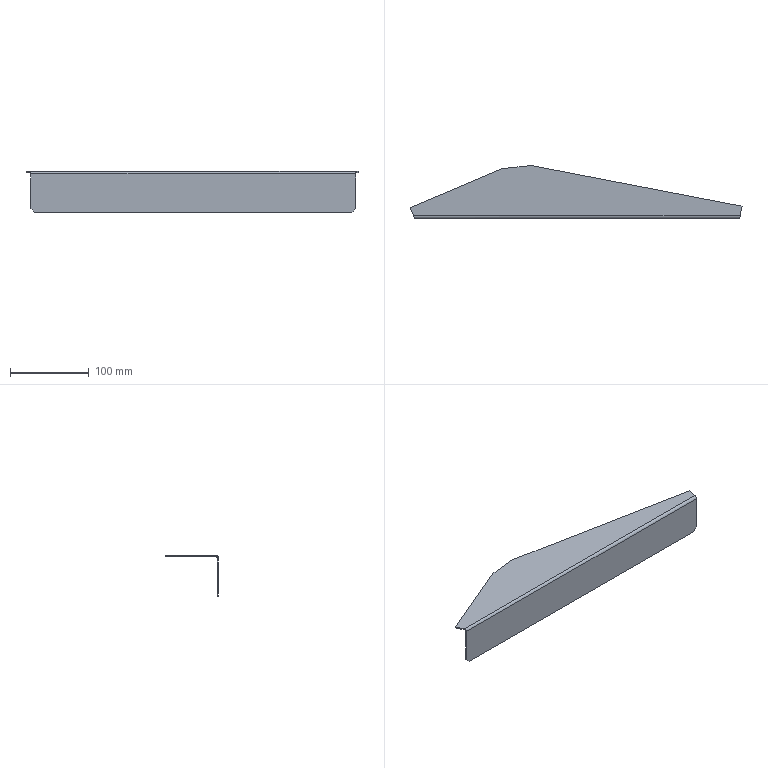Part | SolidWorks | features Chamfer 1, Fillet 1, FlatPattern 1, ICE 1, SMBaseFlange 1, SheetMetal 1 | 1 solid | 24 faces | box 421 x 66.98 x 52 mm | volume 61109 mm3 | plane 14 | spline 6 | cylinder 4 | commonest cylinder face diameters 4 x2 3 x1 6.2 x1
STEP:
#1=CARTESIAN_POINT('',(-56.796,66.969,-1.6));
#2=VERTEX_POINT('',#1);
#3=CARTESIAN_POINT('',(-94.201,63.031,-1.6));
#4=VERTEX_POINT('',#3);
#5=CARTESIAN_POINT('',(200.599,94.063,-1.6));
#6=DIRECTION('',(-0.9945,-0.1047,0.));
#7=VECTOR('',#6,1000.);
#8=LINE('',#5,#7);
#9=EDGE_CURVE('',#2,#4,#8,.T.);
#10=ORIENTED_EDGE('',*,*,#9,.F.);
#11=CARTESIAN_POINT('',(-56.208,66.944,-1.6));
#12=VERTEX_POINT('',#11);
#13=CARTESIAN_POINT('',(-56.587,64.98,-1.6));
#14=DIRECTION('',(0.,0.,-1.));
#15=DIRECTION('',(1.,0.,0.));
#16=AXIS2_PLACEMENT_3D('',#13,#14,#15);
#17=CIRCLE('',#16,2.);
#18=EDGE_CURVE('',#2,#12,#17,.T.);
#19=ORIENTED_EDGE('',*,*,#18,.T.);
#20=CARTESIAN_POINT('',(210.5,15.5,-1.6));
#21=VERTEX_POINT('',#20);
#22=CARTESIAN_POINT('',(213.382,14.944,-1.6));
#23=DIRECTION('',(-0.9819,0.1894,0.));
#24=VECTOR('',#23,1000.);
#25=LINE('',#22,#24);
#26=EDGE_CURVE('',#21,#12,#25,.T.);
#27=ORIENTED_EDGE('',*,*,#26,.F.);
#28=CARTESIAN_POINT('',(208.1,3.1,-1.6));
#29=VERTEX_POINT('',#28);
#30=CARTESIAN_POINT('',(200.008,-38.711,-1.6));
#31=DIRECTION('',(-0.19,-0.9818,0.));
#32=VECTOR('',#31,1000.);
#33=LINE('',#30,#32);
#34=EDGE_CURVE('',#21,#29,#33,.T.);
#35=ORIENTED_EDGE('',*,*,#34,.T.);
#36=CARTESIAN_POINT('',(-205.871,3.1,-1.6));
#37=VERTEX_POINT('',#36);
#38=CARTESIAN_POINT('',(210.5,3.1,-1.6));
#39=DIRECTION('',(-1.,0.,0.));
#40=VECTOR('',#39,1000.);
#41=LINE('',#38,#40);
#42=EDGE_CURVE('',#29,#37,#41,.T.);
#43=ORIENTED_EDGE('',*,*,#42,.T.);
#44=CARTESIAN_POINT('',(-210.5,13.563,-1.6));
#45=VERTEX_POINT('',#44);
#46=CARTESIAN_POINT('',(-136.58,-153.537,-1.6));
#47=DIRECTION('',(-0.4046,0.9145,0.));
#48=VECTOR('',#47,1000.);
#49=LINE('',#46,#48);
#50=EDGE_CURVE('',#37,#45,#49,.T.);
#51=ORIENTED_EDGE('',*,*,#50,.T.);
#52=CARTESIAN_POINT('',(-94.776,62.882,-1.6));
#53=VERTEX_POINT('',#52);
#54=CARTESIAN_POINT('',(140.896,163.321,-1.6));
#55=DIRECTION('',(-0.9199,-0.3921,0.));
#56=VECTOR('',#55,1000.);
#57=LINE('',#54,#56);
#58=EDGE_CURVE('',#53,#45,#57,.T.);
#59=ORIENTED_EDGE('',*,*,#58,.F.);
#60=CARTESIAN_POINT('',(-93.992,61.042,-1.6));
#61=DIRECTION('',(0.,0.,-1.));
#62=DIRECTION('',(1.,0.,0.));
#63=AXIS2_PLACEMENT_3D('',#60,#61,#62);
#64=CIRCLE('',#63,2.);
#65=EDGE_CURVE('',#53,#4,#64,.T.);
#66=ORIENTED_EDGE('',*,*,#65,.T.);
#67=EDGE_LOOP('',(#10,#19,#27,#35,#43,#51,#59,#66));
#68=FACE_OUTER_BOUND('',#67,.T.);
#69=CARTESIAN_POINT('',(210.5,0.,-1.6));
#70=DIRECTION('',(0.,0.,1.));
#71=DIRECTION('',(1.,0.,0.));
#72=AXIS2_PLACEMENT_3D('',#69,#70,#71);
#73=PLANE('',#72);
#74=ADVANCED_FACE('',(#68),#73,.F.);
#75=CARTESIAN_POINT('',(210.5,15.5,0.));
#76=VERTEX_POINT('',#75);
#77=CARTESIAN_POINT('',(-56.208,66.944,0.));
#78=VERTEX_POINT('',#77);
#79=CARTESIAN_POINT('',(213.382,14.944,0.));
#80=DIRECTION('',(-0.9819,0.1894,0.));
#81=VECTOR('',#80,1000.);
#82=LINE('',#79,#81);
#83=EDGE_CURVE('',#76,#78,#82,.T.);
#84=ORIENTED_EDGE('',*,*,#83,.T.);
#85=CARTESIAN_POINT('',(-56.796,66.969,0.));
#86=VERTEX_POINT('',#85);
#87=CARTESIAN_POINT('',(-56.587,64.98,0.));
#88=DIRECTION('',(0.,0.,1.));
#89=DIRECTION('',(1.,0.,0.));
#90=AXIS2_PLACEMENT_3D('',#87,#88,#89);
#91=CIRCLE('',#90,2.);
#92=EDGE_CURVE('',#78,#86,#91,.T.);
#93=ORIENTED_EDGE('',*,*,#92,.T.);
#94=CARTESIAN_POINT('',(-94.201,63.031,0.));
#95=VERTEX_POINT('',#94);
#96=CARTESIAN_POINT('',(200.599,94.063,0.));
#97=DIRECTION('',(-0.9945,-0.1047,0.));
#98=VECTOR('',#97,1000.);
#99=LINE('',#96,#98);
#100=EDGE_CURVE('',#86,#95,#99,.T.);
#101=ORIENTED_EDGE('',*,*,#100,.T.);
#102=CARTESIAN_POINT('',(-94.776,62.882,0.));
#103=VERTEX_POINT('',#102);
#104=CARTESIAN_POINT('',(-93.992,61.042,0.));
#105=DIRECTION('',(0.,0.,1.));
#106=DIRECTION('',(1.,0.,0.));
#107=AXIS2_PLACEMENT_3D('',#104,#105,#106);
#108=CIRCLE('',#107,2.);
#109=EDGE_CURVE('',#95,#103,#108,.T.);
#110=ORIENTED_EDGE('',*,*,#109,.T.);
#111=CARTESIAN_POINT('',(-210.5,13.563,0.));
#112=VERTEX_POINT('',#111);
#113=CARTESIAN_POINT('',(140.896,163.321,0.));
#114=DIRECTION('',(-0.9199,-0.3921,0.));
#115=VECTOR('',#114,1000.);
#116=LINE('',#113,#115);
#117=EDGE_CURVE('',#103,#112,#116,.T.);
#118=ORIENTED_EDGE('',*,*,#117,.T.);
#119=CARTESIAN_POINT('',(-205.871,3.1,0.));
#120=VERTEX_POINT('',#119);
#121=CARTESIAN_POINT('',(-136.58,-153.537,0.));
#122=DIRECTION('',(-0.4046,0.9145,0.));
#123=VECTOR('',#122,1000.);
#124=LINE('',#121,#123);
#125=EDGE_CURVE('',#120,#112,#124,.T.);
#126=ORIENTED_EDGE('',*,*,#125,.F.);
#127=CARTESIAN_POINT('',(208.1,3.1,0.));
#128=VERTEX_POINT('',#127);
#129=CARTESIAN_POINT('',(210.5,3.1,0.));
#130=DIRECTION('',(-1.,0.,0.));
#131=VECTOR('',#130,1000.);
#132=LINE('',#129,#131);
#133=EDGE_CURVE('',#128,#120,#132,.T.);
#134=ORIENTED_EDGE('',*,*,#133,.F.);
#135=CARTESIAN_POINT('',(200.008,-38.711,0.));
#136=DIRECTION('',(-0.19,-0.9818,0.));
#137=VECTOR('',#136,1000.);
#138=LINE('',#135,#137);
#139=EDGE_CURVE('',#76,#128,#138,.T.);
#140=ORIENTED_EDGE('',*,*,#139,.F.);
#141=EDGE_LOOP('',(#84,#93,#101,#110,#118,#126,#134,#140));
#142=FACE_OUTER_BOUND('',#141,.T.);
#143=CARTESIAN_POINT('',(210.5,0.,0.));
#144=DIRECTION('',(0.,0.,1.));
#145=DIRECTION('',(1.,0.,0.));
#146=AXIS2_PLACEMENT_3D('',#143,#144,#145);
#147=PLANE('',#146);
#148=ADVANCED_FACE('',(#142),#147,.T.);
#149=CARTESIAN_POINT('',(207.529,0.09941,-2.321));
#150=VERTEX_POINT('',#149);
#151=CARTESIAN_POINT('',(207.604,0.4379,-1.512));
#152=VERTEX_POINT('',#151);
#153=CARTESIAN_POINT('',(207.529,0.09941,-2.321));
#154=CARTESIAN_POINT('',(207.554,0.1731,-2.037));
#155=CARTESIAN_POINT('',(207.579,0.2875,-1.764));
#156=CARTESIAN_POINT('',(207.604,0.4379,-1.512));
#157=B_SPLINE_CURVE_WITH_KNOTS('',3,(#153,#154,#155,#156),.UNSPECIFIED.,.F.,.F.,(4,4),(0.,1.),.UNSPECIFIED.);
#158=EDGE_CURVE('',#150,#152,#157,.T.);
#159=ORIENTED_EDGE('',*,*,#158,.T.);
#160=CARTESIAN_POINT('',(207.604,0.4379,-1.512));
#161=CARTESIAN_POINT('',(207.645,0.5759,-1.28));
#162=CARTESIAN_POINT('',(207.686,0.7407,-1.072));
#163=CARTESIAN_POINT('',(207.748,1.026,-0.7918));
#164=CARTESIAN_POINT('',(207.769,1.129,-0.7036));
#165=CARTESIAN_POINT('',(207.811,1.343,-0.5427));
#166=CARTESIAN_POINT('',(207.831,1.454,-0.4697));
#167=CARTESIAN_POINT('',(207.893,1.8,-0.273));
#168=CARTESIAN_POINT('',(207.935,2.052,-0.1703));
#169=CARTESIAN_POINT('',(208.017,2.567,-0.03455));
#170=CARTESIAN_POINT('',(208.058,2.831,0.));
#171=CARTESIAN_POINT('',(208.1,3.1,0.));
#172=B_SPLINE_CURVE_WITH_KNOTS('',3,(#160,#161,#162,#163,#164,#165,#166,#167,#168,#169,#170,#171),.UNSPECIFIED.,.F.,.F.,(4,2,2,2,2,4),(0.,0.0008063,0.001209,0.001613,0.002419,0.003225),.UNSPECIFIED.);
#173=EDGE_CURVE('',#152,#128,#172,.T.);
#174=ORIENTED_EDGE('',*,*,#173,.T.);
#175=ORIENTED_EDGE('',*,*,#133,.T.);
#176=CARTESIAN_POINT('',(-204.644,0.2873,-1.797));
#177=VERTEX_POINT('',#176);
#178=CARTESIAN_POINT('',(-205.871,3.1,0.));
#179=CARTESIAN_POINT('',(-205.746,2.812,0.));
#180=CARTESIAN_POINT('',(-205.626,2.529,-0.03947));
#181=CARTESIAN_POINT('',(-205.45,2.113,-0.1577));
#182=CARTESIAN_POINT('',(-205.391,1.975,-0.2075));
#183=CARTESIAN_POINT('',(-205.278,1.71,-0.3255));
#184=CARTESIAN_POINT('',(-205.223,1.582,-0.3934));
#185=CARTESIAN_POINT('',(-205.117,1.335,-0.5473));
#186=CARTESIAN_POINT('',(-205.065,1.217,-0.6333));
#187=CARTESIAN_POINT('',(-204.965,0.9901,-0.824));
#188=CARTESIAN_POINT('',(-204.916,0.8826,-0.9286));
#189=CARTESIAN_POINT('',(-204.826,0.6848,-1.151));
#190=CARTESIAN_POINT('',(-204.784,0.5937,-1.269));
#191=CARTESIAN_POINT('',(-204.707,0.4277,-1.522));
#192=CARTESIAN_POINT('',(-204.672,0.3524,-1.656));
#193=CARTESIAN_POINT('',(-204.644,0.2873,-1.797));
#194=B_SPLINE_CURVE_WITH_KNOTS('',3,(#178,#179,#180,#181,#182,#183,#184,#185,#186,#187,#188,#189,#190,#191,#192,#193),.UNSPECIFIED.,.F.,.F.,(4,2,2,2,2,2,2,4),(0.,0.0009293,0.001394,0.001859,0.002323,0.002788,0.003253,0.003717),.UNSPECIFIED.);
#195=EDGE_CURVE('',#120,#177,#194,.T.);
#196=ORIENTED_EDGE('',*,*,#195,.T.);
#197=CARTESIAN_POINT('',(-204.552,0.07575,-2.419));
#198=VERTEX_POINT('',#197);
#199=CARTESIAN_POINT('',(-204.644,0.2873,-1.797));
#200=CARTESIAN_POINT('',(-204.613,0.195,-1.996));
#201=CARTESIAN_POINT('',(-204.583,0.124,-2.205));
#202=CARTESIAN_POINT('',(-204.552,0.07575,-2.419));
#203=B_SPLINE_CURVE_WITH_KNOTS('',3,(#199,#200,#201,#202),.UNSPECIFIED.,.F.,.F.,(4,4),(0.,1.),.UNSPECIFIED.);
#204=EDGE_CURVE('',#177,#198,#203,.T.);
#205=ORIENTED_EDGE('',*,*,#204,.T.);
#206=CARTESIAN_POINT('',(-204.5,0.,-3.1));
#207=VERTEX_POINT('',#206);
#208=CARTESIAN_POINT('',(-204.552,0.07575,-2.419));
#209=CARTESIAN_POINT('',(-204.535,0.02546,-2.642));
#210=CARTESIAN_POINT('',(-204.517,0.,-2.871));
#211=CARTESIAN_POINT('',(-204.5,0.,-3.1));
#212=B_SPLINE_CURVE_WITH_KNOTS('',3,(#208,#209,#210,#211),.UNSPECIFIED.,.F.,.F.,(4,4),(0.,1.),.UNSPECIFIED.);
#213=EDGE_CURVE('',#198,#207,#212,.T.);
#214=ORIENTED_EDGE('',*,*,#213,.T.);
#215=CARTESIAN_POINT('',(207.5,0.,-3.1));
#216=VERTEX_POINT('',#215);
#217=CARTESIAN_POINT('',(210.5,0.,-3.1));
#218=DIRECTION('',(-1.,0.,0.));
#219=VECTOR('',#218,1000.);
#220=LINE('',#217,#219);
#221=EDGE_CURVE('',#216,#207,#220,.T.);
#222=ORIENTED_EDGE('',*,*,#221,.F.);
#223=CARTESIAN_POINT('',(207.5,0.,-3.1));
#224=CARTESIAN_POINT('',(207.51,0.,-2.838));
#225=CARTESIAN_POINT('',(207.519,0.03349,-2.575));
#226=CARTESIAN_POINT('',(207.529,0.09941,-2.321));
#227=B_SPLINE_CURVE_WITH_KNOTS('',3,(#223,#224,#225,#226),.UNSPECIFIED.,.F.,.F.,(4,4),(0.,1.),.UNSPECIFIED.);
#228=EDGE_CURVE('',#216,#150,#227,.T.);
#229=ORIENTED_EDGE('',*,*,#228,.T.);
#230=EDGE_LOOP('',(#159,#174,#175,#196,#205,#214,#222,#229));
#231=FACE_OUTER_BOUND('',#230,.T.);
#232=CARTESIAN_POINT('',(210.5,3.1,-3.1));
#233=DIRECTION('',(-1.,0.,0.));
#234=DIRECTION('',(0.,0.,1.));
#235=AXIS2_PLACEMENT_3D('',#232,#233,#234);
#236=CYLINDRICAL_SURFACE('',#235,3.1);
#237=ADVANCED_FACE('',(#231),#236,.T.);
#238=CARTESIAN_POINT('',(202.5,0.,-52.));
#239=VERTEX_POINT('',#238);
#240=CARTESIAN_POINT('',(-199.5,0.,-52.));
#241=VERTEX_POINT('',#240);
#242=CARTESIAN_POINT('',(210.5,0.,-52.));
#243=DIRECTION('',(-1.,0.,0.));
#244=VECTOR('',#243,1000.);
#245=LINE('',#242,#244);
#246=EDGE_CURVE('',#239,#241,#245,.T.);
#247=ORIENTED_EDGE('',*,*,#246,.F.);
#248=CARTESIAN_POINT('',(207.5,0.,-47.));
#249=VERTEX_POINT('',#248);
#250=CARTESIAN_POINT('',(232.5,0.,-22.));
#251=DIRECTION('',(0.7071,0.,0.7071));
#252=VECTOR('',#251,1000.);
#253=LINE('',#250,#252);
#254=EDGE_CURVE('',#239,#249,#253,.T.);
#255=ORIENTED_EDGE('',*,*,#254,.T.);
#256=CARTESIAN_POINT('',(207.5,0.,-52.));
#257=DIRECTION('',(0.,0.,1.));
#258=VECTOR('',#257,1000.);
#259=LINE('',#256,#258);
#260=EDGE_CURVE('',#249,#216,#259,.T.);
#261=ORIENTED_EDGE('',*,*,#260,.T.);
#262=ORIENTED_EDGE('',*,*,#221,.T.);
#263=CARTESIAN_POINT('',(-204.5,0.,-47.));
#264=VERTEX_POINT('',#263);
#265=CARTESIAN_POINT('',(-204.5,0.,-52.));
#266=DIRECTION('',(0.,0.,1.));
#267=VECTOR('',#266,1000.);
#268=LINE('',#265,#267);
#269=EDGE_CURVE('',#264,#207,#268,.T.);
#270=ORIENTED_EDGE('',*,*,#269,.F.);
#271=CARTESIAN_POINT('',(-20.5,0.,-231.));
#272=DIRECTION('',(0.7071,0.,-0.7071));
#273=VECTOR('',#272,1000.);
#274=LINE('',#271,#273);
#275=EDGE_CURVE('',#264,#241,#274,.T.);
#276=ORIENTED_EDGE('',*,*,#275,.T.);
#277=EDGE_LOOP('',(#247,#255,#261,#262,#270,#276));
#278=FACE_OUTER_BOUND('',#277,.T.);
#279=CARTESIAN_POINT('',(210.5,0.,0.));
#280=DIRECTION('',(0.,-1.,0.));
#281=DIRECTION('',(0.,0.,-1.));
#282=AXIS2_PLACEMENT_3D('',#279,#280,#281);
#283=PLANE('',#282);
#284=ADVANCED_FACE('',(#278),#283,.T.);
#285=CARTESIAN_POINT('',(202.5,1.6,-52.));
#286=VERTEX_POINT('',#285);
#287=CARTESIAN_POINT('',(-199.5,1.6,-52.));
#288=VERTEX_POINT('',#287);
#289=CARTESIAN_POINT('',(210.5,1.6,-52.));
#290=DIRECTION('',(-1.,0.,0.));
#291=VECTOR('',#290,1000.);
#292=LINE('',#289,#291);
#293=EDGE_CURVE('',#286,#288,#292,.T.);
#294=ORIENTED_EDGE('',*,*,#293,.F.);
#295=CARTESIAN_POINT('',(202.5,1.6,-52.));
#296=DIRECTION('',(0.,-1.,0.));
#297=VECTOR('',#296,1000.);
#298=LINE('',#295,#297);
#299=EDGE_CURVE('',#286,#239,#298,.T.);
#300=ORIENTED_EDGE('',*,*,#299,.T.);
#301=ORIENTED_EDGE('',*,*,#246,.T.);
#302=CARTESIAN_POINT('',(-199.5,1.6,-52.));
#303=DIRECTION('',(0.,1.,0.));
#304=VECTOR('',#303,1000.);
#305=LINE('',#302,#304);
#306=EDGE_CURVE('',#241,#288,#305,.T.);
#307=ORIENTED_EDGE('',*,*,#306,.T.);
#308=EDGE_LOOP('',(#294,#300,#301,#307));
#309=FACE_OUTER_BOUND('',#308,.T.);
#310=CARTESIAN_POINT('',(210.5,1.6,-52.));
#311=DIRECTION('',(0.,0.,-1.));
#312=DIRECTION('',(0.,1.,0.));
#313=AXIS2_PLACEMENT_3D('',#310,#311,#312);
#314=PLANE('',#313);
#315=ADVANCED_FACE('',(#309),#314,.T.);
#316=CARTESIAN_POINT('',(207.5,1.6,-47.));
#317=VERTEX_POINT('',#316);
#318=CARTESIAN_POINT('',(207.5,1.6,-3.1));
#319=VERTEX_POINT('',#318);
#320=CARTESIAN_POINT('',(207.5,1.6,0.));
#321=DIRECTION('',(0.,0.,1.));
#322=VECTOR('',#321,1000.);
#323=LINE('',#320,#322);
#324=EDGE_CURVE('',#317,#319,#323,.T.);
#325=ORIENTED_EDGE('',*,*,#324,.F.);
#326=CARTESIAN_POINT('',(207.5,1.6,-47.));
#327=DIRECTION('',(-0.7071,0.,-0.7071));
#328=VECTOR('',#327,1000.);
#329=LINE('',#326,#328);
#330=EDGE_CURVE('',#317,#286,#329,.T.);
#331=ORIENTED_EDGE('',*,*,#330,.T.);
#332=ORIENTED_EDGE('',*,*,#293,.T.);
#333=CARTESIAN_POINT('',(-204.5,1.6,-47.));
#334=VERTEX_POINT('',#333);
#335=CARTESIAN_POINT('',(-199.5,1.6,-52.));
#336=DIRECTION('',(-0.7071,0.,0.7071));
#337=VECTOR('',#336,1000.);
#338=LINE('',#335,#337);
#339=EDGE_CURVE('',#288,#334,#338,.T.);
#340=ORIENTED_EDGE('',*,*,#339,.T.);
#341=CARTESIAN_POINT('',(-204.5,1.6,-3.1));
#342=VERTEX_POINT('',#341);
#343=CARTESIAN_POINT('',(-204.5,1.6,0.));
#344=DIRECTION('',(0.,0.,1.));
#345=VECTOR('',#344,1000.);
#346=LINE('',#343,#345);
#347=EDGE_CURVE('',#334,#342,#346,.T.);
#348=ORIENTED_EDGE('',*,*,#347,.T.);
#349=CARTESIAN_POINT('',(210.5,1.6,-3.1));
#350=DIRECTION('',(-1.,0.,0.));
#351=VECTOR('',#350,1000.);
#352=LINE('',#349,#351);
#353=EDGE_CURVE('',#319,#342,#352,.T.);
#354=ORIENTED_EDGE('',*,*,#353,.F.);
#355=EDGE_LOOP('',(#325,#331,#332,#340,#348,#354));
#356=FACE_OUTER_BOUND('',#355,.T.);
#357=CARTESIAN_POINT('',(210.5,1.6,0.));
#358=DIRECTION('',(0.,-1.,0.));
#359=DIRECTION('',(0.,0.,-1.));
#360=AXIS2_PLACEMENT_3D('',#357,#358,#359);
#361=PLANE('',#360);
#362=ADVANCED_FACE('',(#356),#361,.F.);
#363=CARTESIAN_POINT('',(207.604,1.812,-2.331));
#364=VERTEX_POINT('',#363);
#365=CARTESIAN_POINT('',(207.604,1.812,-2.331));
#366=CARTESIAN_POINT('',(207.645,1.879,-2.22));
#367=CARTESIAN_POINT('',(207.686,1.958,-2.119));
#368=CARTESIAN_POINT('',(207.769,2.142,-1.938));
#369=CARTESIAN_POINT('',(207.811,2.247,-1.859));
#370=CARTESIAN_POINT('',(207.893,2.471,-1.732));
#371=CARTESIAN_POINT('',(207.934,2.592,-1.683));
#372=CARTESIAN_POINT('',(208.017,2.842,-1.617));
#373=CARTESIAN_POINT('',(208.058,2.97,-1.6));
#374=CARTESIAN_POINT('',(208.1,3.1,-1.6));
#375=B_SPLINE_CURVE_WITH_KNOTS('',3,(#365,#366,#367,#368,#369,#370,#371,#372,#373,#374),.UNSPECIFIED.,.F.,.F.,(4,2,2,2,4),(0.000000002,0.0004046,0.0008091,0.001214,0.001618),.UNSPECIFIED.);
#376=EDGE_CURVE('',#364,#29,#375,.T.);
#377=ORIENTED_EDGE('',*,*,#376,.F.);
#378=CARTESIAN_POINT('',(207.529,1.648,-2.723));
#379=VERTEX_POINT('',#378);
#380=CARTESIAN_POINT('',(207.529,1.648,-2.723));
#381=CARTESIAN_POINT('',(207.554,1.684,-2.586));
#382=CARTESIAN_POINT('',(207.579,1.739,-2.453));
#383=CARTESIAN_POINT('',(207.604,1.812,-2.331));
#384=B_SPLINE_CURVE_WITH_KNOTS('',3,(#380,#381,#382,#383),.UNSPECIFIED.,.F.,.F.,(4,4),(0.000005952,1.),.UNSPECIFIED.);
#385=EDGE_CURVE('',#379,#364,#384,.T.);
#386=ORIENTED_EDGE('',*,*,#385,.F.);
#387=CARTESIAN_POINT('',(207.5,1.6,-3.1));
#388=CARTESIAN_POINT('',(207.51,1.6,-2.973));
#389=CARTESIAN_POINT('',(207.519,1.616,-2.846));
#390=CARTESIAN_POINT('',(207.529,1.648,-2.723));
#391=B_SPLINE_CURVE_WITH_KNOTS('',3,(#387,#388,#389,#390),.UNSPECIFIED.,.F.,.F.,(4,4),(0.,1.),.UNSPECIFIED.);
#392=EDGE_CURVE('',#319,#379,#391,.T.);
#393=ORIENTED_EDGE('',*,*,#392,.F.);
#394=ORIENTED_EDGE('',*,*,#353,.T.);
#395=CARTESIAN_POINT('',(-204.552,1.637,-2.77));
#396=VERTEX_POINT('',#395);
#397=CARTESIAN_POINT('',(-204.552,1.637,-2.77));
#398=CARTESIAN_POINT('',(-204.535,1.612,-2.878));
#399=CARTESIAN_POINT('',(-204.517,1.6,-2.989));
#400=CARTESIAN_POINT('',(-204.5,1.6,-3.1));
#401=B_SPLINE_CURVE_WITH_KNOTS('',3,(#397,#398,#399,#400),.UNSPECIFIED.,.F.,.F.,(4,4),(0.000005695,1.),.UNSPECIFIED.);
#402=EDGE_CURVE('',#396,#342,#401,.T.);
#403=ORIENTED_EDGE('',*,*,#402,.F.);
#404=CARTESIAN_POINT('',(-204.644,1.739,-2.469));
#405=VERTEX_POINT('',#404);
#406=CARTESIAN_POINT('',(-204.644,1.739,-2.469));
#407=CARTESIAN_POINT('',(-204.613,1.694,-2.566));
#408=CARTESIAN_POINT('',(-204.583,1.66,-2.667));
#409=CARTESIAN_POINT('',(-204.552,1.637,-2.77));
#410=B_SPLINE_CURVE_WITH_KNOTS('',3,(#406,#407,#408,#409),.UNSPECIFIED.,.F.,.F.,(4,4),(0.,1.),.UNSPECIFIED.);
#411=EDGE_CURVE('',#405,#396,#410,.T.);
#412=ORIENTED_EDGE('',*,*,#411,.F.);
#413=CARTESIAN_POINT('',(-205.871,3.1,-1.6));
#414=CARTESIAN_POINT('',(-205.753,2.968,-1.6));
#415=CARTESIAN_POINT('',(-205.637,2.837,-1.617));
#416=CARTESIAN_POINT('',(-205.411,2.578,-1.687));
#417=CARTESIAN_POINT('',(-205.299,2.45,-1.741));
#418=CARTESIAN_POINT('',(-205.086,2.211,-1.884));
#419=CARTESIAN_POINT('',(-204.983,2.098,-1.974));
#420=CARTESIAN_POINT('',(-204.793,1.896,-2.193));
#421=CARTESIAN_POINT('',(-204.707,1.809,-2.317));
#422=CARTESIAN_POINT('',(-204.644,1.739,-2.469));
#423=B_SPLINE_CURVE_WITH_KNOTS('',3,(#413,#414,#415,#416,#417,#418,#419,#420,#421,#422),.UNSPECIFIED.,.F.,.F.,(4,2,2,2,4),(0.,0.0005259,0.001052,0.001578,0.002104),.UNSPECIFIED.);
#424=EDGE_CURVE('',#37,#405,#423,.T.);
#425=ORIENTED_EDGE('',*,*,#424,.F.);
#426=ORIENTED_EDGE('',*,*,#42,.F.);
#427=EDGE_LOOP('',(#377,#386,#393,#394,#403,#412,#425,#426));
#428=FACE_OUTER_BOUND('',#427,.T.);
#429=CARTESIAN_POINT('',(210.5,3.1,-3.1));
#430=DIRECTION('',(-1.,0.,0.));
#431=DIRECTION('',(0.,0.,1.));
#432=AXIS2_PLACEMENT_3D('',#429,#430,#431);
#433=CYLINDRICAL_SURFACE('',#432,1.5);
#434=ADVANCED_FACE('',(#428),#433,.F.);
#435=CARTESIAN_POINT('',(-204.552,0.8484,-2.593));
#436=DIRECTION('',(0.,-0.9756,0.2197));
#437=VECTOR('',#436,1000.);
#438=LINE('',#435,#437);
#439=EDGE_CURVE('',#396,#198,#438,.T.);
#440=ORIENTED_EDGE('',*,*,#439,.F.);
#441=ORIENTED_EDGE('',*,*,#402,.T.);
#442=CARTESIAN_POINT('',(-204.5,0.,-3.1));
#443=DIRECTION('',(0.,1.,0.));
#444=VECTOR('',#443,1000.);
#445=LINE('',#442,#444);
#446=EDGE_CURVE('',#207,#342,#445,.T.);
#447=ORIENTED_EDGE('',*,*,#446,.F.);
#448=ORIENTED_EDGE('',*,*,#213,.F.);
#449=EDGE_LOOP('',(#440,#441,#447,#448));
#450=FACE_OUTER_BOUND('',#449,.T.);
#451=CARTESIAN_POINT('',(-204.552,0.06014,-2.415));
#452=CARTESIAN_POINT('',(-204.535,0.009586,-2.64));
#453=CARTESIAN_POINT('',(-204.517,-0.016,-2.87));
#454=CARTESIAN_POINT('',(-204.5,-0.016,-3.1));
#455=CARTESIAN_POINT('',(-204.552,0.07575,-2.419));
#456=CARTESIAN_POINT('',(-204.535,0.02545,-2.642));
#457=CARTESIAN_POINT('',(-204.517,0.,-2.871));
#458=CARTESIAN_POINT('',(-204.5,0.,-3.1));
#459=CARTESIAN_POINT('',(-204.552,1.637,-2.77));
#460=CARTESIAN_POINT('',(-204.535,1.612,-2.878));
#461=CARTESIAN_POINT('',(-204.517,1.6,-2.989));
#462=CARTESIAN_POINT('',(-204.5,1.6,-3.1));
#463=B_SPLINE_SURFACE_WITH_KNOTS('',1,3,((#451,#452,#453,#454),(#455,#456,#457,#458),(#459,#460,#461,#462)),.UNSPECIFIED.,.F.,.F.,.F.,(2,1,2),(4,4),(-0.01,0.,1.),(0.,1.),.UNSPECIFIED.);
#464=ADVANCED_FACE('',(#450),#463,.T.);
#465=CARTESIAN_POINT('',(-204.644,1.006,-2.13));
#466=DIRECTION('',(0.,-0.9073,0.4204));
#467=VECTOR('',#466,1000.);
#468=LINE('',#465,#467);
#469=EDGE_CURVE('',#405,#177,#468,.T.);
#470=ORIENTED_EDGE('',*,*,#469,.F.);
#471=ORIENTED_EDGE('',*,*,#411,.T.);
#472=ORIENTED_EDGE('',*,*,#439,.T.);
#473=ORIENTED_EDGE('',*,*,#204,.F.);
#474=EDGE_LOOP('',(#470,#471,#472,#473));
#475=FACE_OUTER_BOUND('',#474,.T.);
#476=CARTESIAN_POINT('',(-204.644,0.2727,-1.79));
#477=CARTESIAN_POINT('',(-204.613,0.18,-1.99));
#478=CARTESIAN_POINT('',(-204.583,0.1086,-2.2));
#479=CARTESIAN_POINT('',(-204.552,0.06014,-2.415));
#480=CARTESIAN_POINT('',(-204.644,0.2873,-1.797));
#481=CARTESIAN_POINT('',(-204.613,0.195,-1.996));
#482=CARTESIAN_POINT('',(-204.583,0.124,-2.205));
#483=CARTESIAN_POINT('',(-204.552,0.07575,-2.419));
#484=CARTESIAN_POINT('',(-204.644,1.739,-2.469));
#485=CARTESIAN_POINT('',(-204.613,1.694,-2.566));
#486=CARTESIAN_POINT('',(-204.583,1.66,-2.667));
#487=CARTESIAN_POINT('',(-204.552,1.637,-2.77));
#488=B_SPLINE_SURFACE_WITH_KNOTS('',1,3,((#476,#477,#478,#479),(#480,#481,#482,#483),(#484,#485,#486,#487)),.UNSPECIFIED.,.F.,.F.,.F.,(2,1,2),(4,4),(-0.01,0.,1.),(0.,1.),.UNSPECIFIED.);
#489=ADVANCED_FACE('',(#475),#488,.T.);
#490=CARTESIAN_POINT('',(-205.871,3.1,-1.6));
#491=DIRECTION('',(0.,0.,-1.));
#492=VECTOR('',#491,1000.);
#493=LINE('',#490,#492);
#494=EDGE_CURVE('',#120,#37,#493,.T.);
#495=ORIENTED_EDGE('',*,*,#494,.T.);
#496=ORIENTED_EDGE('',*,*,#424,.T.);
#497=ORIENTED_EDGE('',*,*,#469,.T.);
#498=ORIENTED_EDGE('',*,*,#195,.F.);
#499=EDGE_LOOP('',(#495,#496,#497,#498));
#500=FACE_OUTER_BOUND('',#499,.T.);
#501=CARTESIAN_POINT('',(-205.871,3.1,0.016));
#502=CARTESIAN_POINT('',(-205.703,2.712,0.016));
#503=CARTESIAN_POINT('',(-205.552,2.35,-0.05635));
#504=CARTESIAN_POINT('',(-205.282,1.71,-0.2906));
#505=CARTESIAN_POINT('',(-205.163,1.431,-0.4522));
#506=CARTESIAN_POINT('',(-204.958,0.9634,-0.8127));
#507=CARTESIAN_POINT('',(-204.872,0.774,-1.012));
#508=CARTESIAN_POINT('',(-204.734,0.4716,-1.408));
#509=CARTESIAN_POINT('',(-204.681,0.3582,-1.606));
#510=CARTESIAN_POINT('',(-204.644,0.2727,-1.79));
#511=CARTESIAN_POINT('',(-205.871,3.1,0.));
#512=CARTESIAN_POINT('',(-205.703,2.714,0.));
#513=CARTESIAN_POINT('',(-205.552,2.354,-0.07198));
#514=CARTESIAN_POINT('',(-205.282,1.717,-0.3051));
#515=CARTESIAN_POINT('',(-205.163,1.44,-0.4658));
#516=CARTESIAN_POINT('',(-204.958,0.9744,-0.8244));
#517=CARTESIAN_POINT('',(-204.872,0.786,-1.022));
#518=CARTESIAN_POINT('',(-204.734,0.4851,-1.417));
#519=CARTESIAN_POINT('',(-204.681,0.3722,-1.613));
#520=CARTESIAN_POINT('',(-204.644,0.2873,-1.797));
#521=CARTESIAN_POINT('',(-205.871,3.1,-1.6));
#522=CARTESIAN_POINT('',(-205.703,2.914,-1.6));
#523=CARTESIAN_POINT('',(-205.552,2.739,-1.635));
#524=CARTESIAN_POINT('',(-205.282,2.431,-1.748));
#525=CARTESIAN_POINT('',(-205.163,2.297,-1.825));
#526=CARTESIAN_POINT('',(-204.958,2.071,-1.999));
#527=CARTESIAN_POINT('',(-204.872,1.98,-2.095));
#528=CARTESIAN_POINT('',(-204.734,1.835,-2.285));
#529=CARTESIAN_POINT('',(-204.681,1.78,-2.381));
#530=CARTESIAN_POINT('',(-204.644,1.739,-2.469));
#531=CARTESIAN_POINT('',(-205.871,3.1,-1.616));
#532=CARTESIAN_POINT('',(-205.703,2.916,-1.616));
#533=CARTESIAN_POINT('',(-205.552,2.743,-1.651));
#534=CARTESIAN_POINT('',(-205.282,2.438,-1.762));
#535=CARTESIAN_POINT('',(-205.163,2.305,-1.839));
#536=CARTESIAN_POINT('',(-204.958,2.083,-2.011));
#537=CARTESIAN_POINT('',(-204.872,1.992,-2.105));
#538=CARTESIAN_POINT('',(-204.734,1.848,-2.294));
#539=CARTESIAN_POINT('',(-204.681,1.794,-2.388));
#540=CARTESIAN_POINT('',(-204.644,1.754,-2.476));
#541=B_SPLINE_SURFACE_WITH_KNOTS('',1,3,((#501,#502,#503,#504,#505,#506,#507,#508,#509,#510),(#511,#512,#513,#514,#515,#516,#517,#518,#519,#520),(#521,#522,#523,#524,#525,#526,#527,#528,#529,#530),(#531,#532,#533,#534,#535,#536,#537,#538,#539,#540)),.UNSPECIFIED.,.F.,.F.,.F.,(2,1,1,2),(4,2,2,2,4),(-0.01,0.,1.,1.01),(0.,0.25,0.5,0.75,1.),.UNSPECIFIED.);
#542=ADVANCED_FACE('',(#500),#541,.T.);
#543=CARTESIAN_POINT('',(-210.5,13.563,0.));
#544=DIRECTION('',(0.,0.,1.));
#545=VECTOR('',#544,1000.);
#546=LINE('',#543,#545);
#547=EDGE_CURVE('',#45,#112,#546,.T.);
#548=ORIENTED_EDGE('',*,*,#547,.F.);
#549=ORIENTED_EDGE('',*,*,#50,.F.);
#550=ORIENTED_EDGE('',*,*,#494,.F.);
#551=ORIENTED_EDGE('',*,*,#125,.T.);
#552=EDGE_LOOP('',(#548,#549,#550,#551));
#553=FACE_OUTER_BOUND('',#552,.T.);
#554=CARTESIAN_POINT('',(-136.58,-153.537,-1.6));
#555=DIRECTION('',(0.9145,0.4046,0.));
#556=DIRECTION('',(-0.4046,0.9145,0.));
#557=AXIS2_PLACEMENT_3D('',#554,#555,#556);
#558=PLANE('',#557);
#559=ADVANCED_FACE('',(#553),#558,.F.);
#560=ORIENTED_EDGE('',*,*,#347,.F.);
#561=CARTESIAN_POINT('',(-204.5,0.,-47.));
#562=DIRECTION('',(0.,-1.,0.));
#563=VECTOR('',#562,1000.);
#564=LINE('',#561,#563);
#565=EDGE_CURVE('',#334,#264,#564,.T.);
#566=ORIENTED_EDGE('',*,*,#565,.T.);
#567=ORIENTED_EDGE('',*,*,#269,.T.);
#568=ORIENTED_EDGE('',*,*,#446,.T.);
#569=EDGE_LOOP('',(#560,#566,#567,#568));
#570=FACE_OUTER_BOUND('',#569,.T.);
#571=CARTESIAN_POINT('',(-204.5,0.,-52.));
#572=DIRECTION('',(1.,0.,0.));
#573=DIRECTION('',(0.,0.,1.));
#574=AXIS2_PLACEMENT_3D('',#571,#572,#573);
#575=PLANE('',#574);
#576=ADVANCED_FACE('',(#570),#575,.F.);
#577=ORIENTED_EDGE('',*,*,#26,.T.);
#578=CARTESIAN_POINT('',(-56.208,66.944,0.));
#579=DIRECTION('',(0.,0.,1.));
#580=VECTOR('',#579,1000.);
#581=LINE('',#578,#580);
#582=EDGE_CURVE('',#12,#78,#581,.T.);
#583=ORIENTED_EDGE('',*,*,#582,.T.);
#584=ORIENTED_EDGE('',*,*,#83,.F.);
#585=CARTESIAN_POINT('',(210.5,15.5,0.));
#586=DIRECTION('',(0.,0.,1.));
#587=VECTOR('',#586,1000.);
#588=LINE('',#585,#587);
#589=EDGE_CURVE('',#21,#76,#588,.T.);
#590=ORIENTED_EDGE('',*,*,#589,.F.);
#591=EDGE_LOOP('',(#577,#583,#584,#590));
#592=FACE_OUTER_BOUND('',#591,.T.);
#593=CARTESIAN_POINT('',(213.382,14.944,0.));
#594=DIRECTION('',(-0.1894,-0.9819,0.));
#595=DIRECTION('',(-0.9819,0.1894,0.));
#596=AXIS2_PLACEMENT_3D('',#593,#594,#595);
#597=PLANE('',#596);
#598=ADVANCED_FACE('',(#592),#597,.F.);
#599=ORIENTED_EDGE('',*,*,#100,.F.);
#600=CARTESIAN_POINT('',(-56.796,66.969,0.));
#601=DIRECTION('',(0.,0.,-1.));
#602=VECTOR('',#601,1000.);
#603=LINE('',#600,#602);
#604=EDGE_CURVE('',#86,#2,#603,.T.);
#605=ORIENTED_EDGE('',*,*,#604,.T.);
#606=ORIENTED_EDGE('',*,*,#9,.T.);
#607=CARTESIAN_POINT('',(-94.201,63.031,0.));
#608=DIRECTION('',(0.,0.,1.));
#609=VECTOR('',#608,1000.);
#610=LINE('',#607,#609);
#611=EDGE_CURVE('',#4,#95,#610,.T.);
#612=ORIENTED_EDGE('',*,*,#611,.T.);
#613=EDGE_LOOP('',(#599,#605,#606,#612));
#614=FACE_OUTER_BOUND('',#613,.T.);
#615=CARTESIAN_POINT('',(200.599,94.063,0.));
#616=DIRECTION('',(0.1047,-0.9945,0.));
#617=DIRECTION('',(-0.9945,-0.1047,0.));
#618=AXIS2_PLACEMENT_3D('',#615,#616,#617);
#619=PLANE('',#618);
#620=ADVANCED_FACE('',(#614),#619,.F.);
#621=ORIENTED_EDGE('',*,*,#117,.F.);
#622=CARTESIAN_POINT('',(-94.776,62.882,0.));
#623=DIRECTION('',(0.,0.,-1.));
#624=VECTOR('',#623,1000.);
#625=LINE('',#622,#624);
#626=EDGE_CURVE('',#103,#53,#625,.T.);
#627=ORIENTED_EDGE('',*,*,#626,.T.);
#628=ORIENTED_EDGE('',*,*,#58,.T.);
#629=ORIENTED_EDGE('',*,*,#547,.T.);
#630=EDGE_LOOP('',(#621,#627,#628,#629));
#631=FACE_OUTER_BOUND('',#630,.T.);
#632=CARTESIAN_POINT('',(140.896,163.321,0.));
#633=DIRECTION('',(0.3921,-0.9199,0.));
#634=DIRECTION('',(-0.9199,-0.3921,0.));
#635=AXIS2_PLACEMENT_3D('',#632,#633,#634);
#636=PLANE('',#635);
#637=ADVANCED_FACE('',(#631),#636,.F.);
#638=CARTESIAN_POINT('',(207.604,1.118,-1.917));
#639=DIRECTION('',(0.,-0.8588,0.5124));
#640=VECTOR('',#639,1000.);
#641=LINE('',#638,#640);
#642=EDGE_CURVE('',#364,#152,#641,.T.);
#643=ORIENTED_EDGE('',*,*,#642,.F.);
#644=ORIENTED_EDGE('',*,*,#376,.T.);
#645=CARTESIAN_POINT('',(208.1,3.1,0.));
#646=DIRECTION('',(0.,0.,-1.));
#647=VECTOR('',#646,1000.);
#648=LINE('',#645,#647);
#649=EDGE_CURVE('',#128,#29,#648,.T.);
#650=ORIENTED_EDGE('',*,*,#649,.F.);
#651=ORIENTED_EDGE('',*,*,#173,.F.);
#652=EDGE_LOOP('',(#643,#644,#650,#651));
#653=FACE_OUTER_BOUND('',#652,.T.);
#654=CARTESIAN_POINT('',(207.599,0.4076,-1.531));
#655=CARTESIAN_POINT('',(207.6,0.4131,-1.522));
#656=CARTESIAN_POINT('',(207.602,0.4186,-1.513));
#657=CARTESIAN_POINT('',(207.604,0.4241,-1.503));
#658=CARTESIAN_POINT('',(207.686,0.6991,-1.043));
#659=CARTESIAN_POINT('',(207.769,1.095,-0.6552));
#660=CARTESIAN_POINT('',(207.935,2.028,-0.1255));
#661=CARTESIAN_POINT('',(208.017,2.563,0.016));
#662=CARTESIAN_POINT('',(208.1,3.1,0.016));
#663=CARTESIAN_POINT('',(207.599,0.4215,-1.539));
#664=CARTESIAN_POINT('',(207.6,0.4269,-1.53));
#665=CARTESIAN_POINT('',(207.602,0.4324,-1.521));
#666=CARTESIAN_POINT('',(207.604,0.4379,-1.512));
#667=CARTESIAN_POINT('',(207.686,0.7114,-1.053));
#668=CARTESIAN_POINT('',(207.769,1.105,-0.6677));
#669=CARTESIAN_POINT('',(207.935,2.033,-0.1408));
#670=CARTESIAN_POINT('',(208.017,2.566,0.));
#671=CARTESIAN_POINT('',(208.1,3.1,0.));
#672=CARTESIAN_POINT('',(207.599,1.804,-2.345));
#673=CARTESIAN_POINT('',(207.6,1.807,-2.34));
#674=CARTESIAN_POINT('',(207.602,1.809,-2.336));
#675=CARTESIAN_POINT('',(207.604,1.812,-2.331));
#676=CARTESIAN_POINT('',(207.686,1.944,-2.11));
#677=CARTESIAN_POINT('',(207.769,2.135,-1.923));
#678=CARTESIAN_POINT('',(207.935,2.584,-1.668));
#679=CARTESIAN_POINT('',(208.017,2.842,-1.6));
#680=CARTESIAN_POINT('',(208.1,3.1,-1.6));
#681=B_SPLINE_SURFACE_WITH_KNOTS('',1,3,((#654,#655,#656,#657,#658,#659,#660,#661,#662),(#663,#664,#665,#666,#667,#668,#669,#670,#671),(#672,#673,#674,#675,#676,#677,#678,#679,#680)),.UNSPECIFIED.,.F.,.F.,.F.,(2,1,2),(4,3,2,4),(-0.01,0.,1.),(-0.01,0.,0.5,1.),.UNSPECIFIED.);
#682=ADVANCED_FACE('',(#653),#681,.T.);
#683=CARTESIAN_POINT('',(207.529,0.8738,-2.522));
#684=DIRECTION('',(0.,-0.9679,0.2512));
#685=VECTOR('',#684,1000.);
#686=LINE('',#683,#685);
#687=EDGE_CURVE('',#379,#150,#686,.T.);
#688=ORIENTED_EDGE('',*,*,#687,.F.);
#689=ORIENTED_EDGE('',*,*,#385,.T.);
#690=ORIENTED_EDGE('',*,*,#642,.T.);
#691=ORIENTED_EDGE('',*,*,#158,.F.);
#692=EDGE_LOOP('',(#688,#689,#690,#691));
#693=FACE_OUTER_BOUND('',#692,.T.);
#694=CARTESIAN_POINT('',(207.529,0.08392,-2.317));
#695=CARTESIAN_POINT('',(207.554,0.158,-2.032));
#696=CARTESIAN_POINT('',(207.579,0.2729,-1.757));
#697=CARTESIAN_POINT('',(207.604,0.4241,-1.503));
#698=CARTESIAN_POINT('',(207.529,0.09941,-2.321));
#699=CARTESIAN_POINT('',(207.554,0.1732,-2.037));
#700=CARTESIAN_POINT('',(207.579,0.2875,-1.764));
#701=CARTESIAN_POINT('',(207.604,0.4379,-1.512));
#702=CARTESIAN_POINT('',(207.529,1.648,-2.723));
#703=CARTESIAN_POINT('',(207.554,1.684,-2.586));
#704=CARTESIAN_POINT('',(207.579,1.739,-2.453));
#705=CARTESIAN_POINT('',(207.604,1.812,-2.331));
#706=CARTESIAN_POINT('',(207.529,1.664,-2.727));
#707=CARTESIAN_POINT('',(207.554,1.699,-2.591));
#708=CARTESIAN_POINT('',(207.579,1.754,-2.46));
#709=CARTESIAN_POINT('',(207.604,1.826,-2.34));
#710=B_SPLINE_SURFACE_WITH_KNOTS('',1,3,((#694,#695,#696,#697),(#698,#699,#700,#701),(#702,#703,#704,#705),(#706,#707,#708,#709)),.UNSPECIFIED.,.F.,.F.,.F.,(2,1,1,2),(4,4),(-0.01,0.,1.,1.01),(0.000000407,1.),.UNSPECIFIED.);
#711=ADVANCED_FACE('',(#693),#710,.T.);
#712=CARTESIAN_POINT('',(207.5,0.,-3.1));
#713=DIRECTION('',(0.,1.,0.));
#714=VECTOR('',#713,1000.);
#715=LINE('',#712,#714);
#716=EDGE_CURVE('',#216,#319,#715,.T.);
#717=ORIENTED_EDGE('',*,*,#716,.T.);
#718=ORIENTED_EDGE('',*,*,#392,.T.);
#719=ORIENTED_EDGE('',*,*,#687,.T.);
#720=ORIENTED_EDGE('',*,*,#228,.F.);
#721=EDGE_LOOP('',(#717,#718,#719,#720));
#722=FACE_OUTER_BOUND('',#721,.T.);
#723=CARTESIAN_POINT('',(207.5,-0.016,-3.1));
#724=CARTESIAN_POINT('',(207.51,-0.016,-2.836));
#725=CARTESIAN_POINT('',(207.519,0.01766,-2.573));
#726=CARTESIAN_POINT('',(207.529,0.08392,-2.317));
#727=CARTESIAN_POINT('',(207.5,0.,-3.1));
#728=CARTESIAN_POINT('',(207.51,0.,-2.838));
#729=CARTESIAN_POINT('',(207.519,0.03348,-2.575));
#730=CARTESIAN_POINT('',(207.529,0.09941,-2.321));
#731=CARTESIAN_POINT('',(207.5,1.6,-3.1));
#732=CARTESIAN_POINT('',(207.51,1.6,-2.973));
#733=CARTESIAN_POINT('',(207.519,1.616,-2.846));
#734=CARTESIAN_POINT('',(207.529,1.648,-2.723));
#735=B_SPLINE_SURFACE_WITH_KNOTS('',1,3,((#723,#724,#725,#726),(#727,#728,#729,#730),(#731,#732,#733,#734)),.UNSPECIFIED.,.F.,.F.,.F.,(2,1,2),(4,4),(-0.01,0.,1.),(0.,1.),.UNSPECIFIED.);
#736=ADVANCED_FACE('',(#722),#735,.T.);
#737=ORIENTED_EDGE('',*,*,#139,.T.);
#738=ORIENTED_EDGE('',*,*,#649,.T.);
#739=ORIENTED_EDGE('',*,*,#34,.F.);
#740=ORIENTED_EDGE('',*,*,#589,.T.);
#741=EDGE_LOOP('',(#737,#738,#739,#740));
#742=FACE_OUTER_BOUND('',#741,.T.);
#743=CARTESIAN_POINT('',(200.008,-38.711,0.));
#744=DIRECTION('',(-0.9818,0.19,0.));
#745=DIRECTION('',(-0.19,-0.9818,0.));
#746=AXIS2_PLACEMENT_3D('',#743,#744,#745);
#747=PLANE('',#746);
#748=ADVANCED_FACE('',(#742),#747,.F.);
#749=ORIENTED_EDGE('',*,*,#260,.F.);
#750=CARTESIAN_POINT('',(207.5,0.,-47.));
#751=DIRECTION('',(0.,1.,0.));
#752=VECTOR('',#751,1000.);
#753=LINE('',#750,#752);
#754=EDGE_CURVE('',#249,#317,#753,.T.);
#755=ORIENTED_EDGE('',*,*,#754,.T.);
#756=ORIENTED_EDGE('',*,*,#324,.T.);
#757=ORIENTED_EDGE('',*,*,#716,.F.);
#758=EDGE_LOOP('',(#749,#755,#756,#757));
#759=FACE_OUTER_BOUND('',#758,.T.);
#760=CARTESIAN_POINT('',(207.5,0.,-52.));
#761=DIRECTION('',(1.,0.,0.));
#762=DIRECTION('',(0.,0.,1.));
#763=AXIS2_PLACEMENT_3D('',#760,#761,#762);
#764=PLANE('',#763);
#765=ADVANCED_FACE('',(#759),#764,.T.);
#766=ORIENTED_EDGE('',*,*,#254,.F.);
#767=ORIENTED_EDGE('',*,*,#299,.F.);
#768=ORIENTED_EDGE('',*,*,#330,.F.);
#769=ORIENTED_EDGE('',*,*,#754,.F.);
#770=EDGE_LOOP('',(#766,#767,#768,#769));
#771=FACE_OUTER_BOUND('',#770,.T.);
#772=CARTESIAN_POINT('',(207.5,0.,-47.));
#773=DIRECTION('',(-0.7071,0.,0.7071));
#774=DIRECTION('',(0.,1.,0.));
#775=AXIS2_PLACEMENT_3D('',#772,#773,#774);
#776=PLANE('',#775);
#777=ADVANCED_FACE('',(#771),#776,.F.);
#778=ORIENTED_EDGE('',*,*,#275,.F.);
#779=ORIENTED_EDGE('',*,*,#565,.F.);
#780=ORIENTED_EDGE('',*,*,#339,.F.);
#781=ORIENTED_EDGE('',*,*,#306,.F.);
#782=EDGE_LOOP('',(#778,#779,#780,#781));
#783=FACE_OUTER_BOUND('',#782,.T.);
#784=CARTESIAN_POINT('',(-199.5,1.6,-52.));
#785=DIRECTION('',(-0.7071,0.,-0.7071));
#786=DIRECTION('',(0.,-1.,0.));
#787=AXIS2_PLACEMENT_3D('',#784,#785,#786);
#788=PLANE('',#787);
#789=ADVANCED_FACE('',(#783),#788,.T.);
#790=ORIENTED_EDGE('',*,*,#18,.F.);
#791=ORIENTED_EDGE('',*,*,#604,.F.);
#792=ORIENTED_EDGE('',*,*,#92,.F.);
#793=ORIENTED_EDGE('',*,*,#582,.F.);
#794=EDGE_LOOP('',(#790,#791,#792,#793));
#795=FACE_OUTER_BOUND('',#794,.T.);
#796=CARTESIAN_POINT('',(-56.587,64.98,0.));
#797=DIRECTION('',(0.,0.,1.));
#798=DIRECTION('',(1.,0.,0.));
#799=AXIS2_PLACEMENT_3D('',#796,#797,#798);
#800=CYLINDRICAL_SURFACE('',#799,2.);
#801=ADVANCED_FACE('',(#795),#800,.T.);
#802=ORIENTED_EDGE('',*,*,#65,.F.);
#803=ORIENTED_EDGE('',*,*,#626,.F.);
#804=ORIENTED_EDGE('',*,*,#109,.F.);
#805=ORIENTED_EDGE('',*,*,#611,.F.);
#806=EDGE_LOOP('',(#802,#803,#804,#805));
#807=FACE_OUTER_BOUND('',#806,.T.);
#808=CARTESIAN_POINT('',(-93.992,61.042,0.));
#809=DIRECTION('',(0.,0.,1.));
#810=DIRECTION('',(1.,0.,0.));
#811=AXIS2_PLACEMENT_3D('',#808,#809,#810);
#812=CYLINDRICAL_SURFACE('',#811,2.);
#813=ADVANCED_FACE('',(#807),#812,.T.);
#814=CLOSED_SHELL('',(#74,#148,#237,#284,#315,#362,#434,#464,#489,#542,#559,#576,#598,#620,#637,#682,#711,#736,#748,#765,#777,#789,#801,#813));
#815=MANIFOLD_SOLID_BREP('',#814);
#816=CARTESIAN_POINT('',(0.,0.,0.));
#817=DIRECTION('',(0.,0.,1.));
#818=DIRECTION('',(1.,0.,0.));
#819=AXIS2_PLACEMENT_3D('',#816,#817,#818);
#820=(LENGTH_UNIT()NAMED_UNIT(*)SI_UNIT(.MILLI.,.METRE.));
#821=UNCERTAINTY_MEASURE_WITH_UNIT(LENGTH_MEASURE(0.00001),#820,'','');
#822=(NAMED_UNIT(*)PLANE_ANGLE_UNIT()SI_UNIT($,.RADIAN.));
#823=(NAMED_UNIT(*)SI_UNIT($,.STERADIAN.)SOLID_ANGLE_UNIT());
#824=(GEOMETRIC_REPRESENTATION_CONTEXT(3)GLOBAL_UNCERTAINTY_ASSIGNED_CONTEXT((#821))GLOBAL_UNIT_ASSIGNED_CONTEXT((#820,#822,#823))REPRESENTATION_CONTEXT('',''));
#825=ADVANCED_BREP_SHAPE_REPRESENTATION('',(#815,#819),#824);